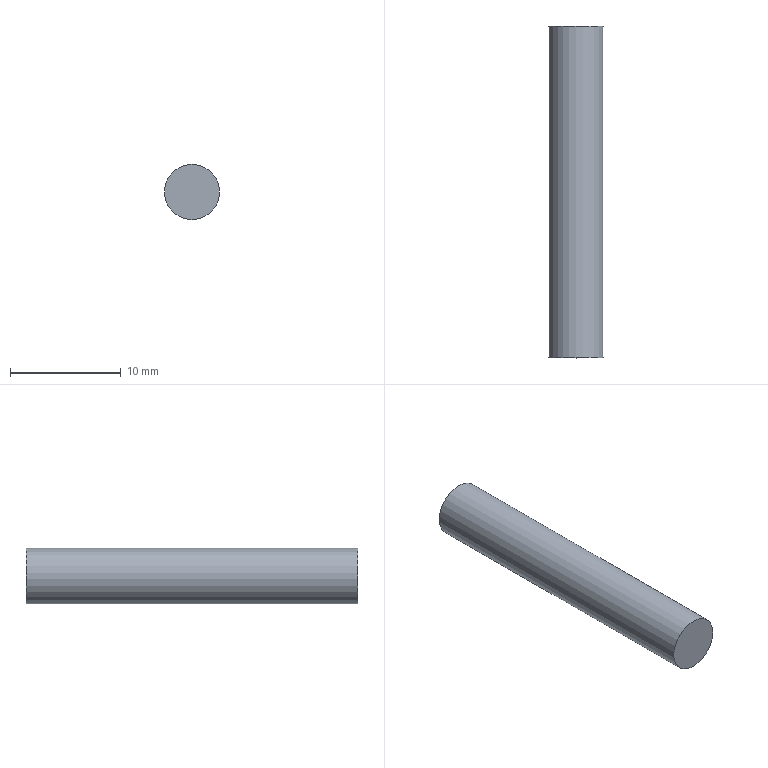Part | STEP file | solid 92 | 1 solid | 3 faces | box 5 x 30 x 5 mm | volume 589.049 mm3 | plane 2 | cylinder 1 | commonest cylinder face diameters 5 x1